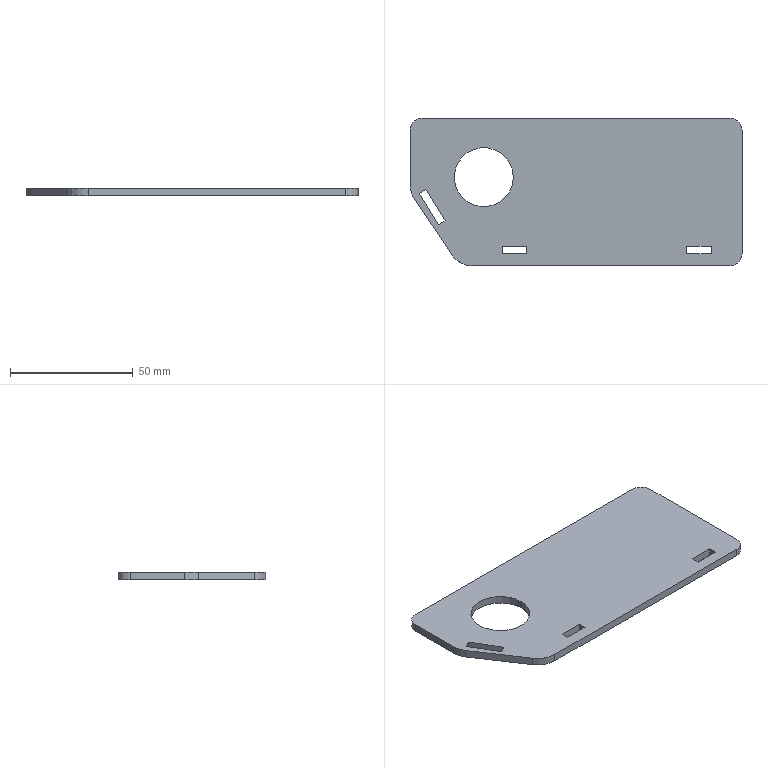Part | SolidWorks | features FlatPattern 1, SMBaseFlange 1, SheetMetal 1 | 1 solid | 26 faces | box 135 x 60 x 3.2 mm | volume 23086 mm3 | plane 19 | cylinder 7 | commonest cylinder face diameters 10 x3 20 x2 24 x2
STEP:
#1=CARTESIAN_POINT('',(19.,28.,3.2));
#2=VERTEX_POINT('',#1);
#3=CARTESIAN_POINT('',(43.,28.,3.2));
#4=VERTEX_POINT('',#3);
#5=CARTESIAN_POINT('',(31.,28.,3.2));
#6=DIRECTION('',(0.,0.,1.));
#7=DIRECTION('',(1.,0.,0.));
#8=AXIS2_PLACEMENT_3D('',#5,#6,#7);
#9=CIRCLE('',#8,12.);
#10=EDGE_CURVE('',#2,#4,#9,.T.);
#11=ORIENTED_EDGE('',*,*,#10,.T.);
#12=CARTESIAN_POINT('',(43.,28.,0.));
#13=VERTEX_POINT('',#12);
#14=CARTESIAN_POINT('',(43.,28.,3.2));
#15=DIRECTION('',(0.,0.,-1.));
#16=VECTOR('',#15,1000.);
#17=LINE('',#14,#16);
#18=EDGE_CURVE('',#4,#13,#17,.T.);
#19=ORIENTED_EDGE('',*,*,#18,.T.);
#20=CARTESIAN_POINT('',(19.,28.,0.));
#21=VERTEX_POINT('',#20);
#22=CARTESIAN_POINT('',(31.,28.,0.));
#23=DIRECTION('',(0.,0.,1.));
#24=DIRECTION('',(1.,0.,0.));
#25=AXIS2_PLACEMENT_3D('',#22,#23,#24);
#26=CIRCLE('',#25,12.);
#27=EDGE_CURVE('',#21,#13,#26,.T.);
#28=ORIENTED_EDGE('',*,*,#27,.F.);
#29=CARTESIAN_POINT('',(19.,28.,3.2));
#30=DIRECTION('',(0.,0.,-1.));
#31=VECTOR('',#30,1000.);
#32=LINE('',#29,#31);
#33=EDGE_CURVE('',#2,#21,#32,.T.);
#34=ORIENTED_EDGE('',*,*,#33,.F.);
#35=EDGE_LOOP('',(#11,#19,#28,#34));
#36=FACE_OUTER_BOUND('',#35,.T.);
#37=CARTESIAN_POINT('',(31.,28.,3.2));
#38=DIRECTION('',(0.,0.,-1.));
#39=DIRECTION('',(-1.,0.,0.));
#40=AXIS2_PLACEMENT_3D('',#37,#38,#39);
#41=CYLINDRICAL_SURFACE('',#40,12.);
#42=ADVANCED_FACE('',(#36),#41,.F.);
#43=CARTESIAN_POINT('',(18.031,-3.547,3.2));
#44=VERTEX_POINT('',#43);
#45=CARTESIAN_POINT('',(26.352,-8.,3.2));
#46=VERTEX_POINT('',#45);
#47=CARTESIAN_POINT('',(26.352,2.,3.2));
#48=DIRECTION('',(0.,0.,1.));
#49=DIRECTION('',(1.,0.,0.));
#50=AXIS2_PLACEMENT_3D('',#47,#48,#49);
#51=CIRCLE('',#50,10.);
#52=EDGE_CURVE('',#44,#46,#51,.T.);
#53=ORIENTED_EDGE('',*,*,#52,.T.);
#54=CARTESIAN_POINT('',(131.,-8.,3.2));
#55=VERTEX_POINT('',#54);
#56=CARTESIAN_POINT('',(26.352,-8.,3.2));
#57=DIRECTION('',(1.,0.,0.));
#58=VECTOR('',#57,1000.);
#59=LINE('',#56,#58);
#60=EDGE_CURVE('',#46,#55,#59,.T.);
#61=ORIENTED_EDGE('',*,*,#60,.T.);
#62=CARTESIAN_POINT('',(136.,-3.,3.2));
#63=VERTEX_POINT('',#62);
#64=CARTESIAN_POINT('',(131.,-3.,3.2));
#65=DIRECTION('',(0.,0.,1.));
#66=DIRECTION('',(-1.,0.,0.));
#67=AXIS2_PLACEMENT_3D('',#64,#65,#66);
#68=CIRCLE('',#67,5.);
#69=EDGE_CURVE('',#55,#63,#68,.T.);
#70=ORIENTED_EDGE('',*,*,#69,.T.);
#71=CARTESIAN_POINT('',(136.,47.,3.2));
#72=VERTEX_POINT('',#71);
#73=CARTESIAN_POINT('',(136.,-3.,3.2));
#74=DIRECTION('',(0.,1.,0.));
#75=VECTOR('',#74,1000.);
#76=LINE('',#73,#75);
#77=EDGE_CURVE('',#63,#72,#76,.T.);
#78=ORIENTED_EDGE('',*,*,#77,.T.);
#79=CARTESIAN_POINT('',(131.,52.,3.2));
#80=VERTEX_POINT('',#79);
#81=CARTESIAN_POINT('',(131.,47.,3.2));
#82=DIRECTION('',(0.,0.,1.));
#83=DIRECTION('',(1.,0.,0.));
#84=AXIS2_PLACEMENT_3D('',#81,#82,#83);
#85=CIRCLE('',#84,5.);
#86=EDGE_CURVE('',#72,#80,#85,.T.);
#87=ORIENTED_EDGE('',*,*,#86,.T.);
#88=CARTESIAN_POINT('',(6.,52.,3.2));
#89=VERTEX_POINT('',#88);
#90=CARTESIAN_POINT('',(131.,52.,3.2));
#91=DIRECTION('',(-1.,0.,0.));
#92=VECTOR('',#91,1000.);
#93=LINE('',#90,#92);
#94=EDGE_CURVE('',#80,#89,#93,.T.);
#95=ORIENTED_EDGE('',*,*,#94,.T.);
#96=CARTESIAN_POINT('',(1.,47.,3.2));
#97=VERTEX_POINT('',#96);
#98=CARTESIAN_POINT('',(6.,47.,3.2));
#99=DIRECTION('',(0.,0.,1.));
#100=DIRECTION('',(1.,0.,0.));
#101=AXIS2_PLACEMENT_3D('',#98,#99,#100);
#102=CIRCLE('',#101,5.);
#103=EDGE_CURVE('',#89,#97,#102,.T.);
#104=ORIENTED_EDGE('',*,*,#103,.T.);
#105=CARTESIAN_POINT('',(1.,25.028,3.2));
#106=VERTEX_POINT('',#105);
#107=CARTESIAN_POINT('',(1.,47.,3.2));
#108=DIRECTION('',(0.,-1.,0.));
#109=VECTOR('',#108,1000.);
#110=LINE('',#107,#109);
#111=EDGE_CURVE('',#97,#106,#110,.T.);
#112=ORIENTED_EDGE('',*,*,#111,.T.);
#113=CARTESIAN_POINT('',(2.679,19.481,3.2));
#114=VERTEX_POINT('',#113);
#115=CARTESIAN_POINT('',(11.,25.028,3.2));
#116=DIRECTION('',(0.,0.,1.));
#117=DIRECTION('',(1.,0.,0.));
#118=AXIS2_PLACEMENT_3D('',#115,#116,#117);
#119=CIRCLE('',#118,10.);
#120=EDGE_CURVE('',#106,#114,#119,.T.);
#121=ORIENTED_EDGE('',*,*,#120,.T.);
#122=CARTESIAN_POINT('',(2.679,19.481,3.2));
#123=DIRECTION('',(0.5547,-0.8321,0.));
#124=VECTOR('',#123,1000.);
#125=LINE('',#122,#124);
#126=EDGE_CURVE('',#114,#44,#125,.T.);
#127=ORIENTED_EDGE('',*,*,#126,.T.);
#128=EDGE_LOOP('',(#53,#61,#70,#78,#87,#95,#104,#112,#121,#127));
#129=FACE_OUTER_BOUND('',#128,.T.);
#130=ORIENTED_EDGE('',*,*,#10,.F.);
#131=CARTESIAN_POINT('',(31.,28.,3.2));
#132=DIRECTION('',(0.,0.,1.));
#133=DIRECTION('',(1.,0.,0.));
#134=AXIS2_PLACEMENT_3D('',#131,#132,#133);
#135=CIRCLE('',#134,12.);
#136=EDGE_CURVE('',#4,#2,#135,.T.);
#137=ORIENTED_EDGE('',*,*,#136,.F.);
#138=EDGE_LOOP('',(#130,#137));
#139=FACE_BOUND('',#138,.T.);
#140=CARTESIAN_POINT('',(15.27,10.261,3.2));
#141=VERTEX_POINT('',#140);
#142=CARTESIAN_POINT('',(7.486,23.082,3.2));
#143=VERTEX_POINT('',#142);
#144=CARTESIAN_POINT('',(7.486,23.082,3.2));
#145=DIRECTION('',(-0.519,0.8548,0.));
#146=VECTOR('',#145,1000.);
#147=LINE('',#144,#146);
#148=EDGE_CURVE('',#141,#143,#147,.T.);
#149=ORIENTED_EDGE('',*,*,#148,.F.);
#150=CARTESIAN_POINT('',(12.535,8.6,3.2));
#151=VERTEX_POINT('',#150);
#152=CARTESIAN_POINT('',(15.27,10.261,3.2));
#153=DIRECTION('',(0.8548,0.519,0.));
#154=VECTOR('',#153,1000.);
#155=LINE('',#152,#154);
#156=EDGE_CURVE('',#151,#141,#155,.T.);
#157=ORIENTED_EDGE('',*,*,#156,.F.);
#158=CARTESIAN_POINT('',(4.75,21.422,3.2));
#159=VERTEX_POINT('',#158);
#160=CARTESIAN_POINT('',(12.535,8.6,3.2));
#161=DIRECTION('',(0.519,-0.8548,0.));
#162=VECTOR('',#161,1000.);
#163=LINE('',#160,#162);
#164=EDGE_CURVE('',#159,#151,#163,.T.);
#165=ORIENTED_EDGE('',*,*,#164,.F.);
#166=CARTESIAN_POINT('',(4.75,21.422,3.2));
#167=DIRECTION('',(-0.8548,-0.519,0.));
#168=VECTOR('',#167,1000.);
#169=LINE('',#166,#168);
#170=EDGE_CURVE('',#143,#159,#169,.T.);
#171=ORIENTED_EDGE('',*,*,#170,.F.);
#172=EDGE_LOOP('',(#149,#157,#165,#171));
#173=FACE_BOUND('',#172,.T.);
#174=CARTESIAN_POINT('',(38.5,-3.2,3.2));
#175=VERTEX_POINT('',#174);
#176=CARTESIAN_POINT('',(48.5,-3.2,3.2));
#177=VERTEX_POINT('',#176);
#178=CARTESIAN_POINT('',(38.5,-3.2,3.2));
#179=DIRECTION('',(1.,0.,0.));
#180=VECTOR('',#179,1000.);
#181=LINE('',#178,#180);
#182=EDGE_CURVE('',#175,#177,#181,.T.);
#183=ORIENTED_EDGE('',*,*,#182,.F.);
#184=CARTESIAN_POINT('',(38.5,0.,3.2));
#185=VERTEX_POINT('',#184);
#186=CARTESIAN_POINT('',(38.5,-3.2,3.2));
#187=DIRECTION('',(0.,-1.,0.));
#188=VECTOR('',#187,1000.);
#189=LINE('',#186,#188);
#190=EDGE_CURVE('',#185,#175,#189,.T.);
#191=ORIENTED_EDGE('',*,*,#190,.F.);
#192=CARTESIAN_POINT('',(48.5,0.,3.2));
#193=VERTEX_POINT('',#192);
#194=CARTESIAN_POINT('',(38.5,0.,3.2));
#195=DIRECTION('',(-1.,0.,0.));
#196=VECTOR('',#195,1000.);
#197=LINE('',#194,#196);
#198=EDGE_CURVE('',#193,#185,#197,.T.);
#199=ORIENTED_EDGE('',*,*,#198,.F.);
#200=CARTESIAN_POINT('',(48.5,-3.2,3.2));
#201=DIRECTION('',(0.,1.,0.));
#202=VECTOR('',#201,1000.);
#203=LINE('',#200,#202);
#204=EDGE_CURVE('',#177,#193,#203,.T.);
#205=ORIENTED_EDGE('',*,*,#204,.F.);
#206=EDGE_LOOP('',(#183,#191,#199,#205));
#207=FACE_BOUND('',#206,.T.);
#208=CARTESIAN_POINT('',(123.5,0.,3.2));
#209=VERTEX_POINT('',#208);
#210=CARTESIAN_POINT('',(113.5,0.,3.2));
#211=VERTEX_POINT('',#210);
#212=CARTESIAN_POINT('',(113.5,0.,3.2));
#213=DIRECTION('',(-1.,0.,0.));
#214=VECTOR('',#213,1000.);
#215=LINE('',#212,#214);
#216=EDGE_CURVE('',#209,#211,#215,.T.);
#217=ORIENTED_EDGE('',*,*,#216,.F.);
#218=CARTESIAN_POINT('',(123.5,-3.2,3.2));
#219=VERTEX_POINT('',#218);
#220=CARTESIAN_POINT('',(123.5,0.,3.2));
#221=DIRECTION('',(0.,1.,0.));
#222=VECTOR('',#221,1000.);
#223=LINE('',#220,#222);
#224=EDGE_CURVE('',#219,#209,#223,.T.);
#225=ORIENTED_EDGE('',*,*,#224,.F.);
#226=CARTESIAN_POINT('',(113.5,-3.2,3.2));
#227=VERTEX_POINT('',#226);
#228=CARTESIAN_POINT('',(123.5,-3.2,3.2));
#229=DIRECTION('',(1.,0.,0.));
#230=VECTOR('',#229,1000.);
#231=LINE('',#228,#230);
#232=EDGE_CURVE('',#227,#219,#231,.T.);
#233=ORIENTED_EDGE('',*,*,#232,.F.);
#234=CARTESIAN_POINT('',(113.5,-3.2,3.2));
#235=DIRECTION('',(0.,-1.,0.));
#236=VECTOR('',#235,1000.);
#237=LINE('',#234,#236);
#238=EDGE_CURVE('',#211,#227,#237,.T.);
#239=ORIENTED_EDGE('',*,*,#238,.F.);
#240=EDGE_LOOP('',(#217,#225,#233,#239));
#241=FACE_BOUND('',#240,.T.);
#242=CARTESIAN_POINT('',(26.352,2.,3.2));
#243=DIRECTION('',(0.,0.,1.));
#244=DIRECTION('',(1.,0.,0.));
#245=AXIS2_PLACEMENT_3D('',#242,#243,#244);
#246=PLANE('',#245);
#247=ADVANCED_FACE('',(#129,#139,#173,#207,#241),#246,.T.);
#248=CARTESIAN_POINT('',(38.5,0.,0.));
#249=VERTEX_POINT('',#248);
#250=CARTESIAN_POINT('',(38.5,-3.2,0.));
#251=VERTEX_POINT('',#250);
#252=CARTESIAN_POINT('',(38.5,-3.2,0.));
#253=DIRECTION('',(0.,-1.,0.));
#254=VECTOR('',#253,1000.);
#255=LINE('',#252,#254);
#256=EDGE_CURVE('',#249,#251,#255,.T.);
#257=ORIENTED_EDGE('',*,*,#256,.T.);
#258=CARTESIAN_POINT('',(48.5,-3.2,0.));
#259=VERTEX_POINT('',#258);
#260=CARTESIAN_POINT('',(38.5,-3.2,0.));
#261=DIRECTION('',(1.,0.,0.));
#262=VECTOR('',#261,1000.);
#263=LINE('',#260,#262);
#264=EDGE_CURVE('',#251,#259,#263,.T.);
#265=ORIENTED_EDGE('',*,*,#264,.T.);
#266=CARTESIAN_POINT('',(48.5,0.,0.));
#267=VERTEX_POINT('',#266);
#268=CARTESIAN_POINT('',(48.5,-3.2,0.));
#269=DIRECTION('',(0.,1.,0.));
#270=VECTOR('',#269,1000.);
#271=LINE('',#268,#270);
#272=EDGE_CURVE('',#259,#267,#271,.T.);
#273=ORIENTED_EDGE('',*,*,#272,.T.);
#274=CARTESIAN_POINT('',(38.5,0.,0.));
#275=DIRECTION('',(-1.,0.,0.));
#276=VECTOR('',#275,1000.);
#277=LINE('',#274,#276);
#278=EDGE_CURVE('',#267,#249,#277,.T.);
#279=ORIENTED_EDGE('',*,*,#278,.T.);
#280=EDGE_LOOP('',(#257,#265,#273,#279));
#281=FACE_BOUND('',#280,.T.);
#282=ORIENTED_EDGE('',*,*,#27,.T.);
#283=CARTESIAN_POINT('',(31.,28.,0.));
#284=DIRECTION('',(0.,0.,1.));
#285=DIRECTION('',(1.,0.,0.));
#286=AXIS2_PLACEMENT_3D('',#283,#284,#285);
#287=CIRCLE('',#286,12.);
#288=EDGE_CURVE('',#13,#21,#287,.T.);
#289=ORIENTED_EDGE('',*,*,#288,.T.);
#290=EDGE_LOOP('',(#282,#289));
#291=FACE_BOUND('',#290,.T.);
#292=CARTESIAN_POINT('',(18.031,-3.547,0.));
#293=VERTEX_POINT('',#292);
#294=CARTESIAN_POINT('',(26.352,-8.,0.));
#295=VERTEX_POINT('',#294);
#296=CARTESIAN_POINT('',(26.352,2.,0.));
#297=DIRECTION('',(0.,0.,1.));
#298=DIRECTION('',(1.,0.,0.));
#299=AXIS2_PLACEMENT_3D('',#296,#297,#298);
#300=CIRCLE('',#299,10.);
#301=EDGE_CURVE('',#293,#295,#300,.T.);
#302=ORIENTED_EDGE('',*,*,#301,.F.);
#303=CARTESIAN_POINT('',(2.679,19.481,0.));
#304=VERTEX_POINT('',#303);
#305=CARTESIAN_POINT('',(2.679,19.481,0.));
#306=DIRECTION('',(0.5547,-0.8321,0.));
#307=VECTOR('',#306,1000.);
#308=LINE('',#305,#307);
#309=EDGE_CURVE('',#304,#293,#308,.T.);
#310=ORIENTED_EDGE('',*,*,#309,.F.);
#311=CARTESIAN_POINT('',(1.,25.028,0.));
#312=VERTEX_POINT('',#311);
#313=CARTESIAN_POINT('',(11.,25.028,0.));
#314=DIRECTION('',(0.,0.,1.));
#315=DIRECTION('',(1.,0.,0.));
#316=AXIS2_PLACEMENT_3D('',#313,#314,#315);
#317=CIRCLE('',#316,10.);
#318=EDGE_CURVE('',#312,#304,#317,.T.);
#319=ORIENTED_EDGE('',*,*,#318,.F.);
#320=CARTESIAN_POINT('',(1.,47.,0.));
#321=VERTEX_POINT('',#320);
#322=CARTESIAN_POINT('',(1.,47.,0.));
#323=DIRECTION('',(0.,-1.,0.));
#324=VECTOR('',#323,1000.);
#325=LINE('',#322,#324);
#326=EDGE_CURVE('',#321,#312,#325,.T.);
#327=ORIENTED_EDGE('',*,*,#326,.F.);
#328=CARTESIAN_POINT('',(6.,52.,0.));
#329=VERTEX_POINT('',#328);
#330=CARTESIAN_POINT('',(6.,47.,0.));
#331=DIRECTION('',(0.,0.,1.));
#332=DIRECTION('',(1.,0.,0.));
#333=AXIS2_PLACEMENT_3D('',#330,#331,#332);
#334=CIRCLE('',#333,5.);
#335=EDGE_CURVE('',#329,#321,#334,.T.);
#336=ORIENTED_EDGE('',*,*,#335,.F.);
#337=CARTESIAN_POINT('',(131.,52.,0.));
#338=VERTEX_POINT('',#337);
#339=CARTESIAN_POINT('',(131.,52.,0.));
#340=DIRECTION('',(-1.,0.,0.));
#341=VECTOR('',#340,1000.);
#342=LINE('',#339,#341);
#343=EDGE_CURVE('',#338,#329,#342,.T.);
#344=ORIENTED_EDGE('',*,*,#343,.F.);
#345=CARTESIAN_POINT('',(136.,47.,0.));
#346=VERTEX_POINT('',#345);
#347=CARTESIAN_POINT('',(131.,47.,0.));
#348=DIRECTION('',(0.,0.,1.));
#349=DIRECTION('',(1.,0.,0.));
#350=AXIS2_PLACEMENT_3D('',#347,#348,#349);
#351=CIRCLE('',#350,5.);
#352=EDGE_CURVE('',#346,#338,#351,.T.);
#353=ORIENTED_EDGE('',*,*,#352,.F.);
#354=CARTESIAN_POINT('',(136.,-3.,0.));
#355=VERTEX_POINT('',#354);
#356=CARTESIAN_POINT('',(136.,-3.,0.));
#357=DIRECTION('',(0.,1.,0.));
#358=VECTOR('',#357,1000.);
#359=LINE('',#356,#358);
#360=EDGE_CURVE('',#355,#346,#359,.T.);
#361=ORIENTED_EDGE('',*,*,#360,.F.);
#362=CARTESIAN_POINT('',(131.,-8.,0.));
#363=VERTEX_POINT('',#362);
#364=CARTESIAN_POINT('',(131.,-3.,0.));
#365=DIRECTION('',(0.,0.,1.));
#366=DIRECTION('',(-1.,0.,0.));
#367=AXIS2_PLACEMENT_3D('',#364,#365,#366);
#368=CIRCLE('',#367,5.);
#369=EDGE_CURVE('',#363,#355,#368,.T.);
#370=ORIENTED_EDGE('',*,*,#369,.F.);
#371=CARTESIAN_POINT('',(26.352,-8.,0.));
#372=DIRECTION('',(1.,0.,0.));
#373=VECTOR('',#372,1000.);
#374=LINE('',#371,#373);
#375=EDGE_CURVE('',#295,#363,#374,.T.);
#376=ORIENTED_EDGE('',*,*,#375,.F.);
#377=EDGE_LOOP('',(#302,#310,#319,#327,#336,#344,#353,#361,#370,#376));
#378=FACE_OUTER_BOUND('',#377,.T.);
#379=CARTESIAN_POINT('',(12.535,8.6,0.));
#380=VERTEX_POINT('',#379);
#381=CARTESIAN_POINT('',(15.27,10.261,0.));
#382=VERTEX_POINT('',#381);
#383=CARTESIAN_POINT('',(15.27,10.261,0.));
#384=DIRECTION('',(0.8548,0.519,0.));
#385=VECTOR('',#384,1000.);
#386=LINE('',#383,#385);
#387=EDGE_CURVE('',#380,#382,#386,.T.);
#388=ORIENTED_EDGE('',*,*,#387,.T.);
#389=CARTESIAN_POINT('',(7.486,23.082,0.));
#390=VERTEX_POINT('',#389);
#391=CARTESIAN_POINT('',(7.486,23.082,0.));
#392=DIRECTION('',(-0.519,0.8548,0.));
#393=VECTOR('',#392,1000.);
#394=LINE('',#391,#393);
#395=EDGE_CURVE('',#382,#390,#394,.T.);
#396=ORIENTED_EDGE('',*,*,#395,.T.);
#397=CARTESIAN_POINT('',(4.75,21.422,0.));
#398=VERTEX_POINT('',#397);
#399=CARTESIAN_POINT('',(4.75,21.422,0.));
#400=DIRECTION('',(-0.8548,-0.519,0.));
#401=VECTOR('',#400,1000.);
#402=LINE('',#399,#401);
#403=EDGE_CURVE('',#390,#398,#402,.T.);
#404=ORIENTED_EDGE('',*,*,#403,.T.);
#405=CARTESIAN_POINT('',(12.535,8.6,0.));
#406=DIRECTION('',(0.519,-0.8548,0.));
#407=VECTOR('',#406,1000.);
#408=LINE('',#405,#407);
#409=EDGE_CURVE('',#398,#380,#408,.T.);
#410=ORIENTED_EDGE('',*,*,#409,.T.);
#411=EDGE_LOOP('',(#388,#396,#404,#410));
#412=FACE_BOUND('',#411,.T.);
#413=CARTESIAN_POINT('',(123.5,-3.2,0.));
#414=VERTEX_POINT('',#413);
#415=CARTESIAN_POINT('',(123.5,0.,0.));
#416=VERTEX_POINT('',#415);
#417=CARTESIAN_POINT('',(123.5,0.,0.));
#418=DIRECTION('',(0.,1.,0.));
#419=VECTOR('',#418,1000.);
#420=LINE('',#417,#419);
#421=EDGE_CURVE('',#414,#416,#420,.T.);
#422=ORIENTED_EDGE('',*,*,#421,.T.);
#423=CARTESIAN_POINT('',(113.5,0.,0.));
#424=VERTEX_POINT('',#423);
#425=CARTESIAN_POINT('',(113.5,0.,0.));
#426=DIRECTION('',(-1.,0.,0.));
#427=VECTOR('',#426,1000.);
#428=LINE('',#425,#427);
#429=EDGE_CURVE('',#416,#424,#428,.T.);
#430=ORIENTED_EDGE('',*,*,#429,.T.);
#431=CARTESIAN_POINT('',(113.5,-3.2,0.));
#432=VERTEX_POINT('',#431);
#433=CARTESIAN_POINT('',(113.5,-3.2,0.));
#434=DIRECTION('',(0.,-1.,0.));
#435=VECTOR('',#434,1000.);
#436=LINE('',#433,#435);
#437=EDGE_CURVE('',#424,#432,#436,.T.);
#438=ORIENTED_EDGE('',*,*,#437,.T.);
#439=CARTESIAN_POINT('',(123.5,-3.2,0.));
#440=DIRECTION('',(1.,0.,0.));
#441=VECTOR('',#440,1000.);
#442=LINE('',#439,#441);
#443=EDGE_CURVE('',#432,#414,#442,.T.);
#444=ORIENTED_EDGE('',*,*,#443,.T.);
#445=EDGE_LOOP('',(#422,#430,#438,#444));
#446=FACE_BOUND('',#445,.T.);
#447=CARTESIAN_POINT('',(26.352,2.,0.));
#448=DIRECTION('',(0.,0.,1.));
#449=DIRECTION('',(1.,0.,0.));
#450=AXIS2_PLACEMENT_3D('',#447,#448,#449);
#451=PLANE('',#450);
#452=ADVANCED_FACE('',(#281,#291,#378,#412,#446),#451,.F.);
#453=ORIENTED_EDGE('',*,*,#301,.T.);
#454=CARTESIAN_POINT('',(26.352,-8.,3.2));
#455=DIRECTION('',(0.,0.,-1.));
#456=VECTOR('',#455,1000.);
#457=LINE('',#454,#456);
#458=EDGE_CURVE('',#46,#295,#457,.T.);
#459=ORIENTED_EDGE('',*,*,#458,.F.);
#460=ORIENTED_EDGE('',*,*,#52,.F.);
#461=CARTESIAN_POINT('',(18.031,-3.547,3.2));
#462=DIRECTION('',(0.,0.,-1.));
#463=VECTOR('',#462,1000.);
#464=LINE('',#461,#463);
#465=EDGE_CURVE('',#44,#293,#464,.T.);
#466=ORIENTED_EDGE('',*,*,#465,.T.);
#467=EDGE_LOOP('',(#453,#459,#460,#466));
#468=FACE_OUTER_BOUND('',#467,.T.);
#469=CARTESIAN_POINT('',(26.352,2.,3.2));
#470=DIRECTION('',(0.,0.,-1.));
#471=DIRECTION('',(-1.,0.,0.));
#472=AXIS2_PLACEMENT_3D('',#469,#470,#471);
#473=CYLINDRICAL_SURFACE('',#472,10.);
#474=ADVANCED_FACE('',(#468),#473,.T.);
#475=ORIENTED_EDGE('',*,*,#375,.T.);
#476=CARTESIAN_POINT('',(131.,-8.,3.2));
#477=DIRECTION('',(0.,0.,-1.));
#478=VECTOR('',#477,1000.);
#479=LINE('',#476,#478);
#480=EDGE_CURVE('',#55,#363,#479,.T.);
#481=ORIENTED_EDGE('',*,*,#480,.F.);
#482=ORIENTED_EDGE('',*,*,#60,.F.);
#483=ORIENTED_EDGE('',*,*,#458,.T.);
#484=EDGE_LOOP('',(#475,#481,#482,#483));
#485=FACE_OUTER_BOUND('',#484,.T.);
#486=CARTESIAN_POINT('',(26.352,-8.,3.2));
#487=DIRECTION('',(0.,1.,0.));
#488=DIRECTION('',(0.,0.,1.));
#489=AXIS2_PLACEMENT_3D('',#486,#487,#488);
#490=PLANE('',#489);
#491=ADVANCED_FACE('',(#485),#490,.F.);
#492=ORIENTED_EDGE('',*,*,#369,.T.);
#493=CARTESIAN_POINT('',(136.,-3.,3.2));
#494=DIRECTION('',(0.,0.,-1.));
#495=VECTOR('',#494,1000.);
#496=LINE('',#493,#495);
#497=EDGE_CURVE('',#63,#355,#496,.T.);
#498=ORIENTED_EDGE('',*,*,#497,.F.);
#499=ORIENTED_EDGE('',*,*,#69,.F.);
#500=ORIENTED_EDGE('',*,*,#480,.T.);
#501=EDGE_LOOP('',(#492,#498,#499,#500));
#502=FACE_OUTER_BOUND('',#501,.T.);
#503=CARTESIAN_POINT('',(131.,-3.,3.2));
#504=DIRECTION('',(0.,0.,-1.));
#505=DIRECTION('',(-1.,0.,0.));
#506=AXIS2_PLACEMENT_3D('',#503,#504,#505);
#507=CYLINDRICAL_SURFACE('',#506,5.);
#508=ADVANCED_FACE('',(#502),#507,.T.);
#509=ORIENTED_EDGE('',*,*,#360,.T.);
#510=CARTESIAN_POINT('',(136.,47.,3.2));
#511=DIRECTION('',(0.,0.,-1.));
#512=VECTOR('',#511,1000.);
#513=LINE('',#510,#512);
#514=EDGE_CURVE('',#72,#346,#513,.T.);
#515=ORIENTED_EDGE('',*,*,#514,.F.);
#516=ORIENTED_EDGE('',*,*,#77,.F.);
#517=ORIENTED_EDGE('',*,*,#497,.T.);
#518=EDGE_LOOP('',(#509,#515,#516,#517));
#519=FACE_OUTER_BOUND('',#518,.T.);
#520=CARTESIAN_POINT('',(136.,-3.,3.2));
#521=DIRECTION('',(-1.,0.,0.));
#522=DIRECTION('',(0.,0.,1.));
#523=AXIS2_PLACEMENT_3D('',#520,#521,#522);
#524=PLANE('',#523);
#525=ADVANCED_FACE('',(#519),#524,.F.);
#526=ORIENTED_EDGE('',*,*,#352,.T.);
#527=CARTESIAN_POINT('',(131.,52.,3.2));
#528=DIRECTION('',(0.,0.,-1.));
#529=VECTOR('',#528,1000.);
#530=LINE('',#527,#529);
#531=EDGE_CURVE('',#80,#338,#530,.T.);
#532=ORIENTED_EDGE('',*,*,#531,.F.);
#533=ORIENTED_EDGE('',*,*,#86,.F.);
#534=ORIENTED_EDGE('',*,*,#514,.T.);
#535=EDGE_LOOP('',(#526,#532,#533,#534));
#536=FACE_OUTER_BOUND('',#535,.T.);
#537=CARTESIAN_POINT('',(131.,47.,3.2));
#538=DIRECTION('',(0.,0.,-1.));
#539=DIRECTION('',(-1.,0.,0.));
#540=AXIS2_PLACEMENT_3D('',#537,#538,#539);
#541=CYLINDRICAL_SURFACE('',#540,5.);
#542=ADVANCED_FACE('',(#536),#541,.T.);
#543=ORIENTED_EDGE('',*,*,#343,.T.);
#544=CARTESIAN_POINT('',(6.,52.,3.2));
#545=DIRECTION('',(0.,0.,-1.));
#546=VECTOR('',#545,1000.);
#547=LINE('',#544,#546);
#548=EDGE_CURVE('',#89,#329,#547,.T.);
#549=ORIENTED_EDGE('',*,*,#548,.F.);
#550=ORIENTED_EDGE('',*,*,#94,.F.);
#551=ORIENTED_EDGE('',*,*,#531,.T.);
#552=EDGE_LOOP('',(#543,#549,#550,#551));
#553=FACE_OUTER_BOUND('',#552,.T.);
#554=CARTESIAN_POINT('',(131.,52.,3.2));
#555=DIRECTION('',(0.,-1.,0.));
#556=DIRECTION('',(1.,0.,0.));
#557=AXIS2_PLACEMENT_3D('',#554,#555,#556);
#558=PLANE('',#557);
#559=ADVANCED_FACE('',(#553),#558,.F.);
#560=ORIENTED_EDGE('',*,*,#335,.T.);
#561=CARTESIAN_POINT('',(1.,47.,3.2));
#562=DIRECTION('',(0.,0.,-1.));
#563=VECTOR('',#562,1000.);
#564=LINE('',#561,#563);
#565=EDGE_CURVE('',#97,#321,#564,.T.);
#566=ORIENTED_EDGE('',*,*,#565,.F.);
#567=ORIENTED_EDGE('',*,*,#103,.F.);
#568=ORIENTED_EDGE('',*,*,#548,.T.);
#569=EDGE_LOOP('',(#560,#566,#567,#568));
#570=FACE_OUTER_BOUND('',#569,.T.);
#571=CARTESIAN_POINT('',(6.,47.,3.2));
#572=DIRECTION('',(0.,0.,-1.));
#573=DIRECTION('',(-1.,0.,0.));
#574=AXIS2_PLACEMENT_3D('',#571,#572,#573);
#575=CYLINDRICAL_SURFACE('',#574,5.);
#576=ADVANCED_FACE('',(#570),#575,.T.);
#577=ORIENTED_EDGE('',*,*,#326,.T.);
#578=CARTESIAN_POINT('',(1.,25.028,3.2));
#579=DIRECTION('',(0.,0.,-1.));
#580=VECTOR('',#579,1000.);
#581=LINE('',#578,#580);
#582=EDGE_CURVE('',#106,#312,#581,.T.);
#583=ORIENTED_EDGE('',*,*,#582,.F.);
#584=ORIENTED_EDGE('',*,*,#111,.F.);
#585=ORIENTED_EDGE('',*,*,#565,.T.);
#586=EDGE_LOOP('',(#577,#583,#584,#585));
#587=FACE_OUTER_BOUND('',#586,.T.);
#588=CARTESIAN_POINT('',(1.,47.,3.2));
#589=DIRECTION('',(1.,0.,0.));
#590=DIRECTION('',(0.,0.,-1.));
#591=AXIS2_PLACEMENT_3D('',#588,#589,#590);
#592=PLANE('',#591);
#593=ADVANCED_FACE('',(#587),#592,.F.);
#594=ORIENTED_EDGE('',*,*,#318,.T.);
#595=CARTESIAN_POINT('',(2.679,19.481,3.2));
#596=DIRECTION('',(0.,0.,-1.));
#597=VECTOR('',#596,1000.);
#598=LINE('',#595,#597);
#599=EDGE_CURVE('',#114,#304,#598,.T.);
#600=ORIENTED_EDGE('',*,*,#599,.F.);
#601=ORIENTED_EDGE('',*,*,#120,.F.);
#602=ORIENTED_EDGE('',*,*,#582,.T.);
#603=EDGE_LOOP('',(#594,#600,#601,#602));
#604=FACE_OUTER_BOUND('',#603,.T.);
#605=CARTESIAN_POINT('',(11.,25.028,3.2));
#606=DIRECTION('',(0.,0.,-1.));
#607=DIRECTION('',(-1.,0.,0.));
#608=AXIS2_PLACEMENT_3D('',#605,#606,#607);
#609=CYLINDRICAL_SURFACE('',#608,10.);
#610=ADVANCED_FACE('',(#604),#609,.T.);
#611=ORIENTED_EDGE('',*,*,#309,.T.);
#612=ORIENTED_EDGE('',*,*,#465,.F.);
#613=ORIENTED_EDGE('',*,*,#126,.F.);
#614=ORIENTED_EDGE('',*,*,#599,.T.);
#615=EDGE_LOOP('',(#611,#612,#613,#614));
#616=FACE_OUTER_BOUND('',#615,.T.);
#617=CARTESIAN_POINT('',(2.679,19.481,3.2));
#618=DIRECTION('',(0.8321,0.5547,0.));
#619=DIRECTION('',(-0.5547,0.8321,0.));
#620=AXIS2_PLACEMENT_3D('',#617,#618,#619);
#621=PLANE('',#620);
#622=ADVANCED_FACE('',(#616),#621,.F.);
#623=ORIENTED_EDGE('',*,*,#18,.F.);
#624=ORIENTED_EDGE('',*,*,#136,.T.);
#625=ORIENTED_EDGE('',*,*,#33,.T.);
#626=ORIENTED_EDGE('',*,*,#288,.F.);
#627=EDGE_LOOP('',(#623,#624,#625,#626));
#628=FACE_OUTER_BOUND('',#627,.T.);
#629=CARTESIAN_POINT('',(31.,28.,3.2));
#630=DIRECTION('',(0.,0.,-1.));
#631=DIRECTION('',(-1.,0.,0.));
#632=AXIS2_PLACEMENT_3D('',#629,#630,#631);
#633=CYLINDRICAL_SURFACE('',#632,12.);
#634=ADVANCED_FACE('',(#628),#633,.F.);
#635=ORIENTED_EDGE('',*,*,#387,.F.);
#636=CARTESIAN_POINT('',(12.535,8.6,3.2));
#637=DIRECTION('',(0.,0.,-1.));
#638=VECTOR('',#637,1000.);
#639=LINE('',#636,#638);
#640=EDGE_CURVE('',#151,#380,#639,.T.);
#641=ORIENTED_EDGE('',*,*,#640,.F.);
#642=ORIENTED_EDGE('',*,*,#156,.T.);
#643=CARTESIAN_POINT('',(15.27,10.261,3.2));
#644=DIRECTION('',(0.,0.,-1.));
#645=VECTOR('',#644,1000.);
#646=LINE('',#643,#645);
#647=EDGE_CURVE('',#141,#382,#646,.T.);
#648=ORIENTED_EDGE('',*,*,#647,.T.);
#649=EDGE_LOOP('',(#635,#641,#642,#648));
#650=FACE_OUTER_BOUND('',#649,.T.);
#651=CARTESIAN_POINT('',(15.27,10.261,3.2));
#652=DIRECTION('',(-0.519,0.8548,0.));
#653=DIRECTION('',(-0.8548,-0.519,0.));
#654=AXIS2_PLACEMENT_3D('',#651,#652,#653);
#655=PLANE('',#654);
#656=ADVANCED_FACE('',(#650),#655,.T.);
#657=ORIENTED_EDGE('',*,*,#395,.F.);
#658=ORIENTED_EDGE('',*,*,#647,.F.);
#659=ORIENTED_EDGE('',*,*,#148,.T.);
#660=CARTESIAN_POINT('',(7.486,23.082,3.2));
#661=DIRECTION('',(0.,0.,-1.));
#662=VECTOR('',#661,1000.);
#663=LINE('',#660,#662);
#664=EDGE_CURVE('',#143,#390,#663,.T.);
#665=ORIENTED_EDGE('',*,*,#664,.T.);
#666=EDGE_LOOP('',(#657,#658,#659,#665));
#667=FACE_OUTER_BOUND('',#666,.T.);
#668=CARTESIAN_POINT('',(7.486,23.082,3.2));
#669=DIRECTION('',(-0.8548,-0.519,0.));
#670=DIRECTION('',(0.519,-0.8548,0.));
#671=AXIS2_PLACEMENT_3D('',#668,#669,#670);
#672=PLANE('',#671);
#673=ADVANCED_FACE('',(#667),#672,.T.);
#674=ORIENTED_EDGE('',*,*,#403,.F.);
#675=ORIENTED_EDGE('',*,*,#664,.F.);
#676=ORIENTED_EDGE('',*,*,#170,.T.);
#677=CARTESIAN_POINT('',(4.75,21.422,3.2));
#678=DIRECTION('',(0.,0.,-1.));
#679=VECTOR('',#678,1000.);
#680=LINE('',#677,#679);
#681=EDGE_CURVE('',#159,#398,#680,.T.);
#682=ORIENTED_EDGE('',*,*,#681,.T.);
#683=EDGE_LOOP('',(#674,#675,#676,#682));
#684=FACE_OUTER_BOUND('',#683,.T.);
#685=CARTESIAN_POINT('',(4.75,21.422,3.2));
#686=DIRECTION('',(0.519,-0.8548,0.));
#687=DIRECTION('',(0.8548,0.519,0.));
#688=AXIS2_PLACEMENT_3D('',#685,#686,#687);
#689=PLANE('',#688);
#690=ADVANCED_FACE('',(#684),#689,.T.);
#691=ORIENTED_EDGE('',*,*,#409,.F.);
#692=ORIENTED_EDGE('',*,*,#681,.F.);
#693=ORIENTED_EDGE('',*,*,#164,.T.);
#694=ORIENTED_EDGE('',*,*,#640,.T.);
#695=EDGE_LOOP('',(#691,#692,#693,#694));
#696=FACE_OUTER_BOUND('',#695,.T.);
#697=CARTESIAN_POINT('',(12.535,8.6,3.2));
#698=DIRECTION('',(0.8548,0.519,0.));
#699=DIRECTION('',(-0.519,0.8548,0.));
#700=AXIS2_PLACEMENT_3D('',#697,#698,#699);
#701=PLANE('',#700);
#702=ADVANCED_FACE('',(#696),#701,.T.);
#703=ORIENTED_EDGE('',*,*,#256,.F.);
#704=CARTESIAN_POINT('',(38.5,0.,3.2));
#705=DIRECTION('',(0.,0.,-1.));
#706=VECTOR('',#705,1000.);
#707=LINE('',#704,#706);
#708=EDGE_CURVE('',#185,#249,#707,.T.);
#709=ORIENTED_EDGE('',*,*,#708,.F.);
#710=ORIENTED_EDGE('',*,*,#190,.T.);
#711=CARTESIAN_POINT('',(38.5,-3.2,3.2));
#712=DIRECTION('',(0.,0.,-1.));
#713=VECTOR('',#712,1000.);
#714=LINE('',#711,#713);
#715=EDGE_CURVE('',#175,#251,#714,.T.);
#716=ORIENTED_EDGE('',*,*,#715,.T.);
#717=EDGE_LOOP('',(#703,#709,#710,#716));
#718=FACE_OUTER_BOUND('',#717,.T.);
#719=CARTESIAN_POINT('',(38.5,-3.2,3.2));
#720=DIRECTION('',(1.,0.,0.));
#721=DIRECTION('',(0.,0.,-1.));
#722=AXIS2_PLACEMENT_3D('',#719,#720,#721);
#723=PLANE('',#722);
#724=ADVANCED_FACE('',(#718),#723,.T.);
#725=ORIENTED_EDGE('',*,*,#264,.F.);
#726=ORIENTED_EDGE('',*,*,#715,.F.);
#727=ORIENTED_EDGE('',*,*,#182,.T.);
#728=CARTESIAN_POINT('',(48.5,-3.2,3.2));
#729=DIRECTION('',(0.,0.,-1.));
#730=VECTOR('',#729,1000.);
#731=LINE('',#728,#730);
#732=EDGE_CURVE('',#177,#259,#731,.T.);
#733=ORIENTED_EDGE('',*,*,#732,.T.);
#734=EDGE_LOOP('',(#725,#726,#727,#733));
#735=FACE_OUTER_BOUND('',#734,.T.);
#736=CARTESIAN_POINT('',(38.5,-3.2,3.2));
#737=DIRECTION('',(0.,1.,0.));
#738=DIRECTION('',(0.,0.,1.));
#739=AXIS2_PLACEMENT_3D('',#736,#737,#738);
#740=PLANE('',#739);
#741=ADVANCED_FACE('',(#735),#740,.T.);
#742=ORIENTED_EDGE('',*,*,#272,.F.);
#743=ORIENTED_EDGE('',*,*,#732,.F.);
#744=ORIENTED_EDGE('',*,*,#204,.T.);
#745=CARTESIAN_POINT('',(48.5,0.,3.2));
#746=DIRECTION('',(0.,0.,-1.));
#747=VECTOR('',#746,1000.);
#748=LINE('',#745,#747);
#749=EDGE_CURVE('',#193,#267,#748,.T.);
#750=ORIENTED_EDGE('',*,*,#749,.T.);
#751=EDGE_LOOP('',(#742,#743,#744,#750));
#752=FACE_OUTER_BOUND('',#751,.T.);
#753=CARTESIAN_POINT('',(48.5,-3.2,3.2));
#754=DIRECTION('',(-1.,0.,0.));
#755=DIRECTION('',(0.,0.,1.));
#756=AXIS2_PLACEMENT_3D('',#753,#754,#755);
#757=PLANE('',#756);
#758=ADVANCED_FACE('',(#752),#757,.T.);
#759=ORIENTED_EDGE('',*,*,#278,.F.);
#760=ORIENTED_EDGE('',*,*,#749,.F.);
#761=ORIENTED_EDGE('',*,*,#198,.T.);
#762=ORIENTED_EDGE('',*,*,#708,.T.);
#763=EDGE_LOOP('',(#759,#760,#761,#762));
#764=FACE_OUTER_BOUND('',#763,.T.);
#765=CARTESIAN_POINT('',(38.5,0.,3.2));
#766=DIRECTION('',(0.,-1.,0.));
#767=DIRECTION('',(0.,0.,-1.));
#768=AXIS2_PLACEMENT_3D('',#765,#766,#767);
#769=PLANE('',#768);
#770=ADVANCED_FACE('',(#764),#769,.T.);
#771=ORIENTED_EDGE('',*,*,#421,.F.);
#772=CARTESIAN_POINT('',(123.5,-3.2,3.2));
#773=DIRECTION('',(0.,0.,-1.));
#774=VECTOR('',#773,1000.);
#775=LINE('',#772,#774);
#776=EDGE_CURVE('',#219,#414,#775,.T.);
#777=ORIENTED_EDGE('',*,*,#776,.F.);
#778=ORIENTED_EDGE('',*,*,#224,.T.);
#779=CARTESIAN_POINT('',(123.5,0.,3.2));
#780=DIRECTION('',(0.,0.,-1.));
#781=VECTOR('',#780,1000.);
#782=LINE('',#779,#781);
#783=EDGE_CURVE('',#209,#416,#782,.T.);
#784=ORIENTED_EDGE('',*,*,#783,.T.);
#785=EDGE_LOOP('',(#771,#777,#778,#784));
#786=FACE_OUTER_BOUND('',#785,.T.);
#787=CARTESIAN_POINT('',(123.5,0.,3.2));
#788=DIRECTION('',(-1.,0.,0.));
#789=DIRECTION('',(0.,0.,1.));
#790=AXIS2_PLACEMENT_3D('',#787,#788,#789);
#791=PLANE('',#790);
#792=ADVANCED_FACE('',(#786),#791,.T.);
#793=ORIENTED_EDGE('',*,*,#429,.F.);
#794=ORIENTED_EDGE('',*,*,#783,.F.);
#795=ORIENTED_EDGE('',*,*,#216,.T.);
#796=CARTESIAN_POINT('',(113.5,0.,3.2));
#797=DIRECTION('',(0.,0.,-1.));
#798=VECTOR('',#797,1000.);
#799=LINE('',#796,#798);
#800=EDGE_CURVE('',#211,#424,#799,.T.);
#801=ORIENTED_EDGE('',*,*,#800,.T.);
#802=EDGE_LOOP('',(#793,#794,#795,#801));
#803=FACE_OUTER_BOUND('',#802,.T.);
#804=CARTESIAN_POINT('',(113.5,0.,3.2));
#805=DIRECTION('',(0.,-1.,0.));
#806=DIRECTION('',(1.,0.,0.));
#807=AXIS2_PLACEMENT_3D('',#804,#805,#806);
#808=PLANE('',#807);
#809=ADVANCED_FACE('',(#803),#808,.T.);
#810=ORIENTED_EDGE('',*,*,#437,.F.);
#811=ORIENTED_EDGE('',*,*,#800,.F.);
#812=ORIENTED_EDGE('',*,*,#238,.T.);
#813=CARTESIAN_POINT('',(113.5,-3.2,3.2));
#814=DIRECTION('',(0.,0.,-1.));
#815=VECTOR('',#814,1000.);
#816=LINE('',#813,#815);
#817=EDGE_CURVE('',#227,#432,#816,.T.);
#818=ORIENTED_EDGE('',*,*,#817,.T.);
#819=EDGE_LOOP('',(#810,#811,#812,#818));
#820=FACE_OUTER_BOUND('',#819,.T.);
#821=CARTESIAN_POINT('',(113.5,-3.2,3.2));
#822=DIRECTION('',(1.,0.,0.));
#823=DIRECTION('',(0.,0.,-1.));
#824=AXIS2_PLACEMENT_3D('',#821,#822,#823);
#825=PLANE('',#824);
#826=ADVANCED_FACE('',(#820),#825,.T.);
#827=ORIENTED_EDGE('',*,*,#443,.F.);
#828=ORIENTED_EDGE('',*,*,#817,.F.);
#829=ORIENTED_EDGE('',*,*,#232,.T.);
#830=ORIENTED_EDGE('',*,*,#776,.T.);
#831=EDGE_LOOP('',(#827,#828,#829,#830));
#832=FACE_OUTER_BOUND('',#831,.T.);
#833=CARTESIAN_POINT('',(123.5,-3.2,3.2));
#834=DIRECTION('',(0.,1.,0.));
#835=DIRECTION('',(0.,0.,1.));
#836=AXIS2_PLACEMENT_3D('',#833,#834,#835);
#837=PLANE('',#836);
#838=ADVANCED_FACE('',(#832),#837,.T.);
#839=CLOSED_SHELL('',(#42,#247,#452,#474,#491,#508,#525,#542,#559,#576,#593,#610,#622,#634,#656,#673,#690,#702,#724,#741,#758,#770,#792,#809,#826,#838));
#840=MANIFOLD_SOLID_BREP('',#839);
#841=CARTESIAN_POINT('',(0.,0.,0.));
#842=DIRECTION('',(0.,0.,1.));
#843=DIRECTION('',(1.,0.,0.));
#844=AXIS2_PLACEMENT_3D('',#841,#842,#843);
#845=(LENGTH_UNIT()NAMED_UNIT(*)SI_UNIT(.MILLI.,.METRE.));
#846=UNCERTAINTY_MEASURE_WITH_UNIT(LENGTH_MEASURE(0.00001),#845,'','');
#847=(NAMED_UNIT(*)PLANE_ANGLE_UNIT()SI_UNIT($,.RADIAN.));
#848=(NAMED_UNIT(*)SI_UNIT($,.STERADIAN.)SOLID_ANGLE_UNIT());
#849=(GEOMETRIC_REPRESENTATION_CONTEXT(3)GLOBAL_UNCERTAINTY_ASSIGNED_CONTEXT((#846))GLOBAL_UNIT_ASSIGNED_CONTEXT((#845,#847,#848))REPRESENTATION_CONTEXT('',''));
#850=ADVANCED_BREP_SHAPE_REPRESENTATION('',(#840,#844),#849);